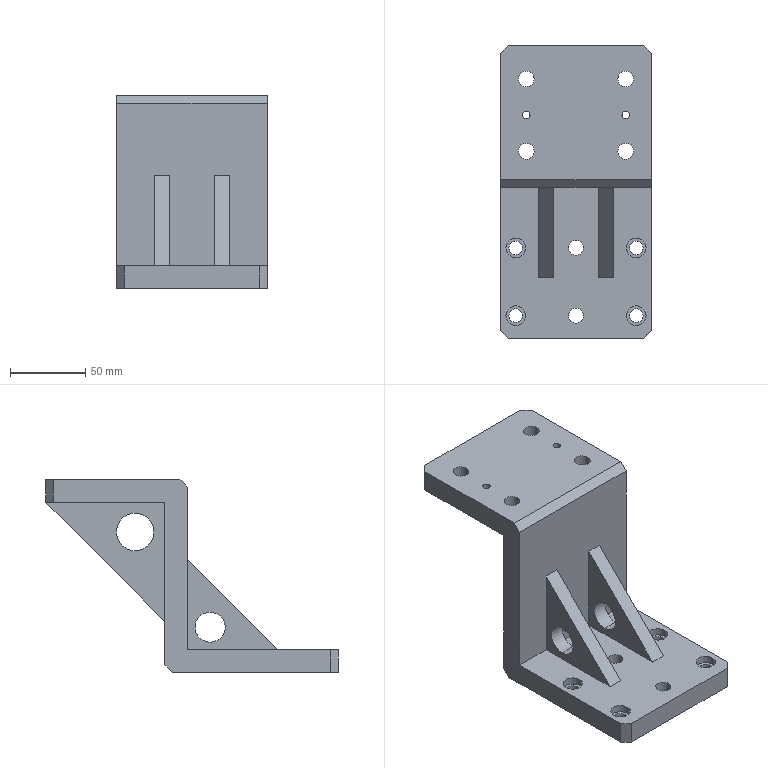Part | SolidWorks | features BaseBody 1 | 1 solid | 80 faces | box 100 x 194 x 128 mm | volume 497627 mm3 | cylinder 46 | plane 34 | commonest cylinder face diameters 9 x8 10.5 x8 13 x8 16 x8 5.01 x4 10.01 x4